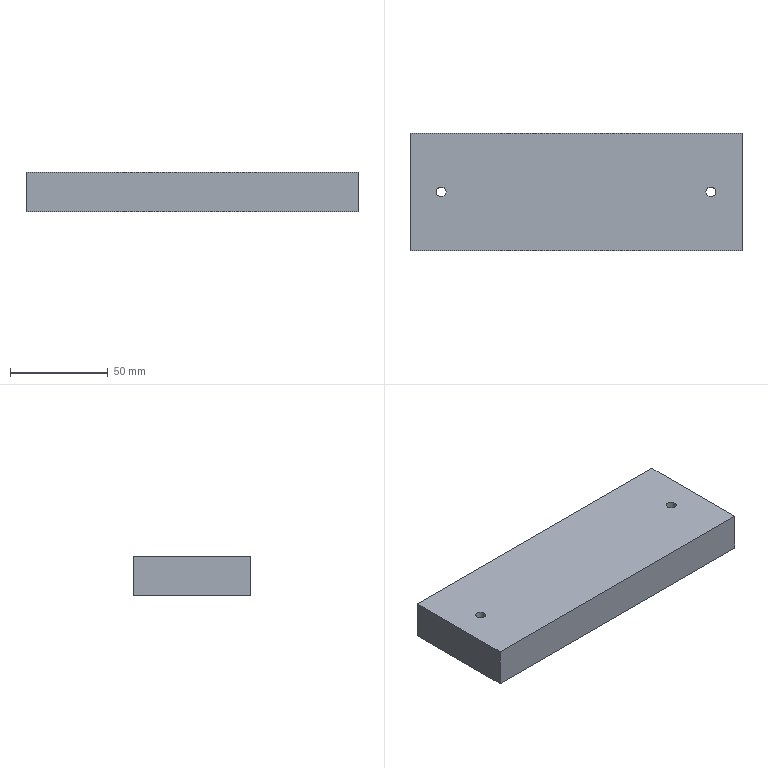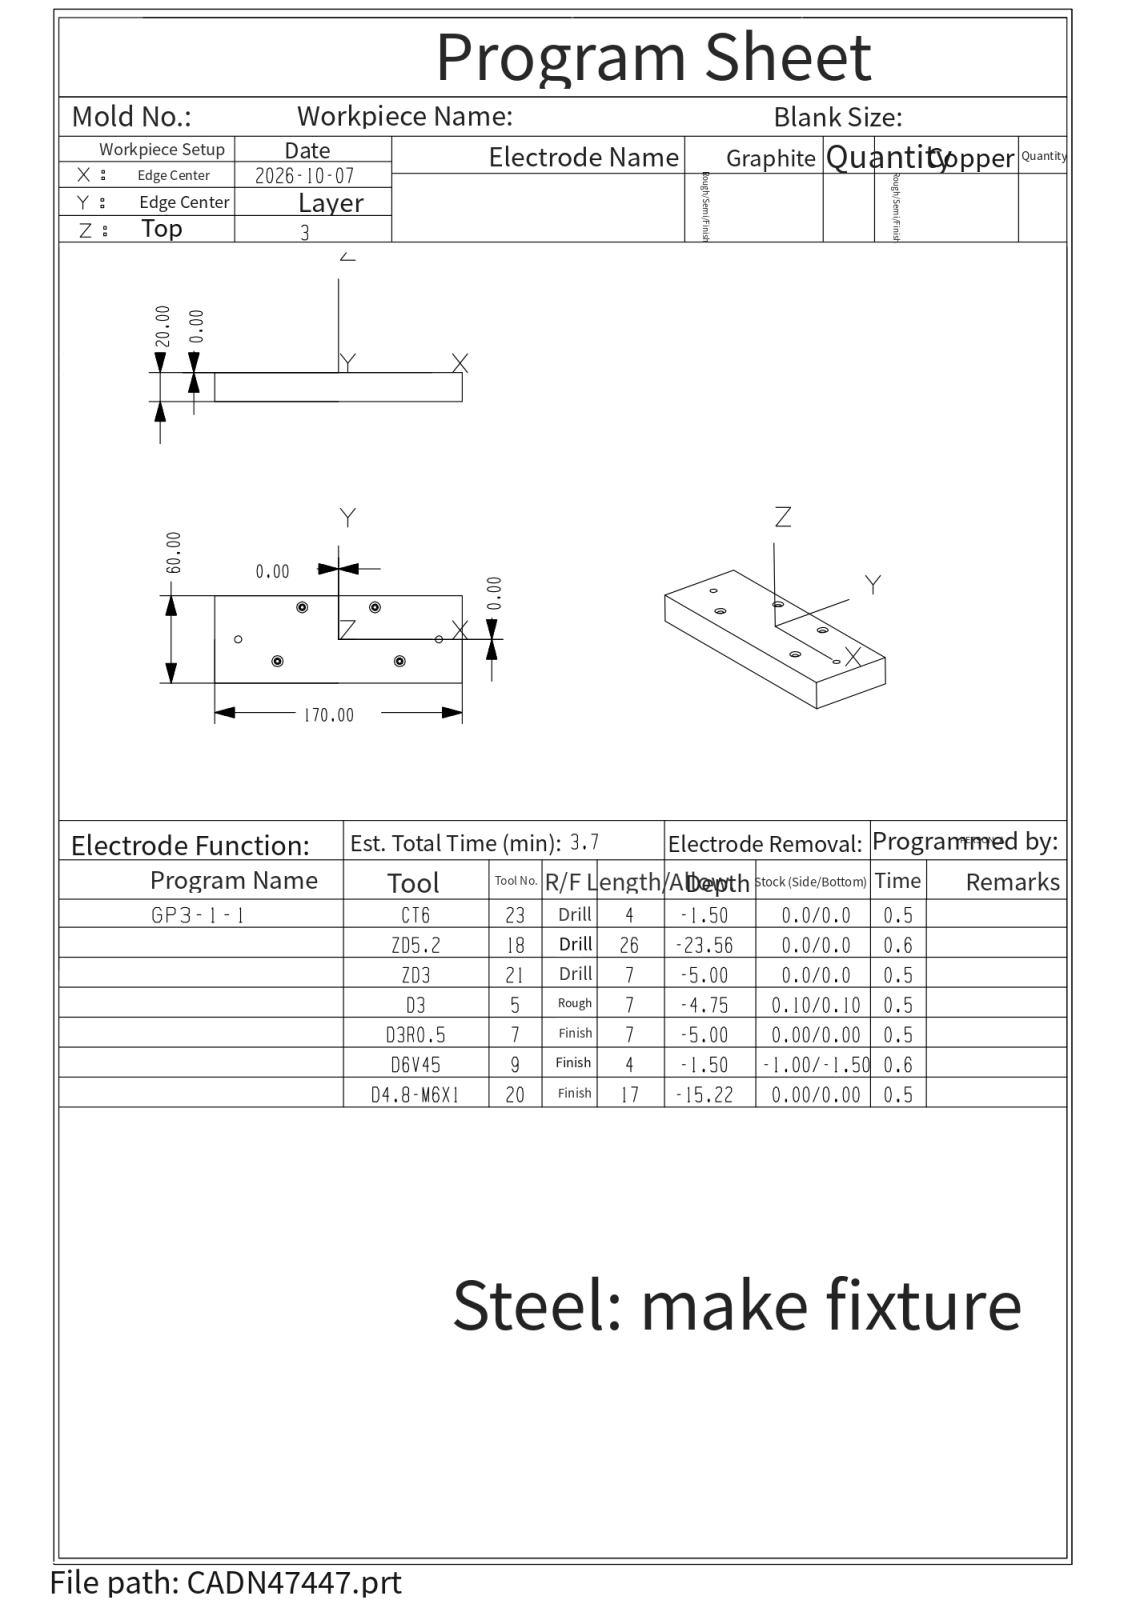NC program | NX | posted by the shop | part box 170 x 60 x 20 mm
Lines 13298 to 14163 of 14163:
T09 M06
T20
( name=D6V45    T=9 )
( XY = -0.50 )
( Z = -1.50 )
G00 G90 G54 X0.0 Y-31.6 S5000 M03
G43 Z10. H09 M08
Z-1.5
G01 X.6 F500.
G03 X0.0 Y-31. I-.6 J0.0
G01 X-84.5 F1000.
G02 X-86. Y-29.5 I0.0 J1.5
G01 Y29.5
G02 X-84.5 Y31. I1.5 J0.0
G01 X84.5
G02 X86. Y29.5 I0.0 J-1.5
G01 Y-29.5
G02 X84.5 Y-31. I-1.5 J0.0
G01 X0.0
G03 X-.6 Y-31.6 I0.0 J-.6
G01 X0.0
G00 Z10.
G00 X68.1 Y0.0 S5000 M03
M08
Z-1.5
G01 Y.6 F500.
G03 X67.5 Y0.0 I0.0 J-.6
I1.5 J0.0 F1000.
X68.1 Y-.6 I.6 J0.0
G01 Y0.0
X67.6
Y.6 F500.
G03 X67. Y0.0 I0.0 J-.6
I2. J0.0 F1000.
X67.6 Y-.6 I.6 J0.0
G01 Y0.0
G00 Z10.
X-69.9
Z-1.5
G01 Y.6 F500.
G03 X-70.5 Y0.0 I0.0 J-.6
I1.5 J0.0 F1000.
X-69.9 Y-.6 I.6 J0.0
G01 Y0.0
X-70.4
Y.6 F500.
G03 X-71. Y0.0 I0.0 J-.6
I2. J0.0 F1000.
X-70.4 Y-.6 I.6 J0.0
G01 Y0.0
G00 Z10.
M05
M09
G91 G28 Z0.0
M01
N07
T20 M06
T23
( name=D4.8-M6X1    T=20 )
( XY = 0.00 )
( Z = -1.50 )
G00 G90 G54 X69. Y0.0 S6000 M03
G43 Z10. H20 M08
Z.218
G01 X69.032 Y.095 F1000.
X69.119 Y.235 Z.174
X69.273 Y.3 Z.131
X69.439 Y.272 Z.087
X69.564 Y.161 Z.044
X69.6 Y0.0 Z0.0
X69.532 Y-.299 Z-.082 F2000.
X69.317 Y-.521 Z-.163
X69.021 Y-.61 Z-.245
X68.719 Y-.542 Z-.326
X68.49 Y-.335 Z-.408
X68.391 Y-.042 Z-.489
X68.449 Y.262 Z-.571
X68.648 Y.498 Z-.652
X68.938 Y.607 Z-.734
X69.243 Y.559 Z-.815
X69.486 Y.369 Z-.897
X69.604 Y.083 Z-.978
X69.567 Y-.224 Z-1.06
X69.385 Y-.473 Z-1.141
X69.104 Y-.601 Z-1.223
X68.796 Y-.575 Z-1.304
X68.54 Y-.401 Z-1.386
X68.403 Y-.124 Z-1.467
X68.419 Y.185 Z-1.549
X68.584 Y.446 Z-1.63
X68.856 Y.593 Z-1.712
X69.165 Y.587 Z-1.793
X69.431 Y.431 Z-1.875
X69.587 Y.165 Z-1.957
X69.593 Y-.144 Z-2.038
X69.446 Y-.416 Z-2.12
X69.185 Y-.581 Z-2.201
X68.876 Y-.597 Z-2.283
X68.599 Y-.46 Z-2.364
X68.425 Y-.204 Z-2.446
X68.399 Y.104 Z-2.527
X68.527 Y.385 Z-2.609
X68.776 Y.567 Z-2.69
X69.083 Y.604 Z-2.772
X69.369 Y.486 Z-2.853
X69.559 Y.243 Z-2.935
X69.607 Y-.062 Z-3.016
X69.498 Y-.352 Z-3.098
X69.262 Y-.551 Z-3.179
X68.958 Y-.609 Z-3.261
X68.665 Y-.51 Z-3.342
X68.458 Y-.281 Z-3.424
X68.39 Y.021 Z-3.505
X68.479 Y.317 Z-3.587
X68.701 Y.532 Z-3.668
X69. Y.61 Z-3.75
X69.299 Y.532 Z-3.832
X69.521 Y.317 Z-3.913
X69.61 Y.021 Z-3.995
X69.542 Y-.281 Z-4.076
X69.335 Y-.51 Z-4.158
X69.042 Y-.609 Z-4.239
X68.738 Y-.551 Z-4.321
X68.502 Y-.352 Z-4.402
X68.393 Y-.062 Z-4.484
X68.441 Y.243 Z-4.565
X68.631 Y.486 Z-4.647
X68.917 Y.604 Z-4.728
X69.224 Y.567 Z-4.81
X69.473 Y.385 Z-4.891
X69.601 Y.104 Z-4.973
X69.575 Y-.204 Z-5.054
X69.401 Y-.46 Z-5.136
X69.124 Y-.597 Z-5.217
X68.815 Y-.581 Z-5.299
X68.554 Y-.416 Z-5.38
X68.407 Y-.144 Z-5.462
X68.413 Y.165 Z-5.543
X68.569 Y.431 Z-5.625
X68.835 Y.587 Z-5.707
X69.144 Y.593 Z-5.788
X69.416 Y.446 Z-5.87
X69.581 Y.185 Z-5.951
X69.597 Y-.124 Z-6.033
X69.46 Y-.401 Z-6.114
X69.204 Y-.575 Z-6.196
X68.896 Y-.601 Z-6.277
X68.615 Y-.473 Z-6.359
X68.433 Y-.224 Z-6.44
X68.396 Y.083 Z-6.522
X68.514 Y.369 Z-6.603
X68.757 Y.559 Z-6.685
X69.062 Y.607 Z-6.766
X69.352 Y.498 Z-6.848
X69.551 Y.262 Z-6.929
X69.609 Y-.042 Z-7.011
X69.51 Y-.335 Z-7.092
X69.281 Y-.542 Z-7.174
X68.979 Y-.61 Z-7.255
X68.683 Y-.521 Z-7.337
X68.468 Y-.299 Z-7.418
X68.39 Y0.0 Z-7.5
X68.468 Y.299 Z-7.582
X68.683 Y.521 Z-7.663
X68.979 Y.61 Z-7.745
X69.281 Y.542 Z-7.826
X69.51 Y.335 Z-7.908
X69.609 Y.042 Z-7.989
X69.551 Y-.262 Z-8.071
X69.352 Y-.498 Z-8.152
X69.062 Y-.607 Z-8.234
X68.757 Y-.559 Z-8.315
X68.514 Y-.369 Z-8.397
X68.396 Y-.083 Z-8.478
X68.433 Y.224 Z-8.56
X68.615 Y.473 Z-8.641
X68.896 Y.601 Z-8.723
X69.204 Y.575 Z-8.804
X69.46 Y.401 Z-8.886
X69.597 Y.124 Z-8.967
X69.581 Y-.185 Z-9.049
X69.416 Y-.446 Z-9.13
X69.144 Y-.593 Z-9.212
X68.835 Y-.587 Z-9.293
X68.569 Y-.431 Z-9.375
X68.413 Y-.165 Z-9.457
X68.407 Y.144 Z-9.538
X68.554 Y.416 Z-9.62
X68.815 Y.581 Z-9.701
X69.124 Y.597 Z-9.783
X69.401 Y.46 Z-9.864
X69.575 Y.204 Z-9.946
X69.601 Y-.104 Z-10.027
X69.473 Y-.385 Z-10.109
X69.224 Y-.567 Z-10.19
X68.917 Y-.604 Z-10.272
X68.631 Y-.486 Z-10.353
X68.441 Y-.243 Z-10.435
X68.393 Y.062 Z-10.516
X68.502 Y.352 Z-10.598
X68.738 Y.551 Z-10.679
X69.042 Y.609 Z-10.761
X69.335 Y.51 Z-10.842
X69.542 Y.281 Z-10.924
X69.61 Y-.021 Z-11.005
X69.521 Y-.317 Z-11.087
X69.299 Y-.532 Z-11.168
X69. Y-.61 Z-11.25
X68.701 Y-.532 Z-11.332
X68.479 Y-.317 Z-11.413
X68.39 Y-.021 Z-11.495
X68.458 Y.281 Z-11.576
X68.665 Y.51 Z-11.658
X68.958 Y.609 Z-11.739
X69.262 Y.551 Z-11.821
X69.498 Y.352 Z-11.902
X69.607 Y.062 Z-11.984
X69.559 Y-.243 Z-12.065
X69.369 Y-.486 Z-12.147
X69.083 Y-.604 Z-12.228
X68.776 Y-.567 Z-12.31
X68.527 Y-.385 Z-12.391
X68.399 Y-.104 Z-12.473
X68.425 Y.204 Z-12.554
X68.599 Y.46 Z-12.636
X68.876 Y.597 Z-12.717
X69.185 Y.581 Z-12.799
X69.446 Y.416 Z-12.88
X69.593 Y.144 Z-12.962
X69.587 Y-.165 Z-13.043
X69.431 Y-.431 Z-13.125
X69.165 Y-.587 Z-13.207
X68.856 Y-.593 Z-13.288
X68.584 Y-.446 Z-13.37
X68.419 Y-.185 Z-13.451
X68.403 Y.124 Z-13.533
X68.54 Y.401 Z-13.614
X68.796 Y.575 Z-13.696
X69.104 Y.601 Z-13.777
X69.385 Y.473 Z-13.859
X69.567 Y.224 Z-13.94
X69.604 Y-.083 Z-14.022
X69.486 Y-.369 Z-14.103
X69.243 Y-.559 Z-14.185
X68.938 Y-.607 Z-14.266
X68.648 Y-.498 Z-14.348
X68.449 Y-.262 Z-14.429
X68.391 Y.042 Z-14.511
X68.49 Y.335 Z-14.592
X68.719 Y.542 Z-14.674
X69.021 Y.61 Z-14.755
X69.317 Y.521 Z-14.837
X69.532 Y.299 Z-14.918
X69.6 Y0.0 Z-15.
X69.564 Y-.161 Z-15.044
X69.439 Y-.272 Z-15.087
X69.273 Y-.3 Z-15.131
X69.119 Y-.235 Z-15.174
X69.032 Y-.095 Z-15.218
X69. Y0.0
G00 Z10.
Z.218
G01 X69.032 Y.095 F1000.
X69.119 Y.235 Z.174
X69.273 Y.3 Z.131
X69.439 Y.272 Z.087
X69.564 Y.161 Z.044
X69.6 Y0.0 Z0.0
X69.532 Y-.299 Z-.082 F2000.
X69.317 Y-.521 Z-.163
X69.021 Y-.61 Z-.245
X68.719 Y-.542 Z-.326
X68.49 Y-.335 Z-.408
X68.391 Y-.042 Z-.489
X68.449 Y.262 Z-.571
X68.648 Y.498 Z-.652
X68.938 Y.607 Z-.734
X69.243 Y.559 Z-.815
X69.486 Y.369 Z-.897
X69.604 Y.083 Z-.978
X69.567 Y-.224 Z-1.06
X69.385 Y-.473 Z-1.141
X69.104 Y-.601 Z-1.223
X68.796 Y-.575 Z-1.304
X68.54 Y-.401 Z-1.386
X68.403 Y-.124 Z-1.467
X68.419 Y.185 Z-1.549
X68.584 Y.446 Z-1.63
X68.856 Y.593 Z-1.712
X69.165 Y.587 Z-1.793
X69.431 Y.431 Z-1.875
X69.587 Y.165 Z-1.957
X69.593 Y-.144 Z-2.038
X69.446 Y-.416 Z-2.12
X69.185 Y-.581 Z-2.201
X68.876 Y-.597 Z-2.283
X68.599 Y-.46 Z-2.364
X68.425 Y-.204 Z-2.446
X68.399 Y.104 Z-2.527
X68.527 Y.385 Z-2.609
X68.776 Y.567 Z-2.69
X69.083 Y.604 Z-2.772
X69.369 Y.486 Z-2.853
X69.559 Y.243 Z-2.935
X69.607 Y-.062 Z-3.016
X69.498 Y-.352 Z-3.098
X69.262 Y-.551 Z-3.179
X68.958 Y-.609 Z-3.261
X68.665 Y-.51 Z-3.342
X68.458 Y-.281 Z-3.424
X68.39 Y.021 Z-3.505
X68.479 Y.317 Z-3.587
X68.701 Y.532 Z-3.668
X69. Y.61 Z-3.75
X69.299 Y.532 Z-3.832
X69.521 Y.317 Z-3.913
X69.61 Y.021 Z-3.995
X69.542 Y-.281 Z-4.076
X69.335 Y-.51 Z-4.158
X69.042 Y-.609 Z-4.239
X68.738 Y-.551 Z-4.321
X68.502 Y-.352 Z-4.402
X68.393 Y-.062 Z-4.484
X68.441 Y.243 Z-4.565
X68.631 Y.486 Z-4.647
X68.917 Y.604 Z-4.728
X69.224 Y.567 Z-4.81
X69.473 Y.385 Z-4.891
X69.601 Y.104 Z-4.973
X69.575 Y-.204 Z-5.054
X69.401 Y-.46 Z-5.136
X69.124 Y-.597 Z-5.217
X68.815 Y-.581 Z-5.299
X68.554 Y-.416 Z-5.38
X68.407 Y-.144 Z-5.462
X68.413 Y.165 Z-5.543
X68.569 Y.431 Z-5.625
X68.835 Y.587 Z-5.707
X69.144 Y.593 Z-5.788
X69.416 Y.446 Z-5.87
X69.581 Y.185 Z-5.951
X69.597 Y-.124 Z-6.033
X69.46 Y-.401 Z-6.114
X69.204 Y-.575 Z-6.196
X68.896 Y-.601 Z-6.277
X68.615 Y-.473 Z-6.359
X68.433 Y-.224 Z-6.44
X68.396 Y.083 Z-6.522
X68.514 Y.369 Z-6.603
X68.757 Y.559 Z-6.685
X69.062 Y.607 Z-6.766
X69.352 Y.498 Z-6.848
X69.551 Y.262 Z-6.929
X69.609 Y-.042 Z-7.011
X69.51 Y-.335 Z-7.092
X69.281 Y-.542 Z-7.174
X68.979 Y-.61 Z-7.255
X68.683 Y-.521 Z-7.337
X68.468 Y-.299 Z-7.418
X68.39 Y0.0 Z-7.5
X68.468 Y.299 Z-7.582
X68.683 Y.521 Z-7.663
X68.979 Y.61 Z-7.745
X69.281 Y.542 Z-7.826
X69.51 Y.335 Z-7.908
X69.609 Y.042 Z-7.989
X69.551 Y-.262 Z-8.071
X69.352 Y-.498 Z-8.152
X69.062 Y-.607 Z-8.234
X68.757 Y-.559 Z-8.315
X68.514 Y-.369 Z-8.397
X68.396 Y-.083 Z-8.478
X68.433 Y.224 Z-8.56
X68.615 Y.473 Z-8.641
X68.896 Y.601 Z-8.723
X69.204 Y.575 Z-8.804
X69.46 Y.401 Z-8.886
X69.597 Y.124 Z-8.967
X69.581 Y-.185 Z-9.049
X69.416 Y-.446 Z-9.13
X69.144 Y-.593 Z-9.212
X68.835 Y-.587 Z-9.293
X68.569 Y-.431 Z-9.375
X68.413 Y-.165 Z-9.457
X68.407 Y.144 Z-9.538
X68.554 Y.416 Z-9.62
X68.815 Y.581 Z-9.701
X69.124 Y.597 Z-9.783
X69.401 Y.46 Z-9.864
X69.575 Y.204 Z-9.946
X69.601 Y-.104 Z-10.027
X69.473 Y-.385 Z-10.109
X69.224 Y-.567 Z-10.19
X68.917 Y-.604 Z-10.272
X68.631 Y-.486 Z-10.353
X68.441 Y-.243 Z-10.435
X68.393 Y.062 Z-10.516
X68.502 Y.352 Z-10.598
X68.738 Y.551 Z-10.679
X69.042 Y.609 Z-10.761
X69.335 Y.51 Z-10.842
X69.542 Y.281 Z-10.924
X69.61 Y-.021 Z-11.005
X69.521 Y-.317 Z-11.087
X69.299 Y-.532 Z-11.168
X69. Y-.61 Z-11.25
X68.701 Y-.532 Z-11.332
X68.479 Y-.317 Z-11.413
X68.39 Y-.021 Z-11.495
X68.458 Y.281 Z-11.576
X68.665 Y.51 Z-11.658
X68.958 Y.609 Z-11.739
X69.262 Y.551 Z-11.821
X69.498 Y.352 Z-11.902
X69.607 Y.062 Z-11.984
X69.559 Y-.243 Z-12.065
X69.369 Y-.486 Z-12.147
X69.083 Y-.604 Z-12.228
X68.776 Y-.567 Z-12.31
X68.527 Y-.385 Z-12.391
X68.399 Y-.104 Z-12.473
X68.425 Y.204 Z-12.554
X68.599 Y.46 Z-12.636
X68.876 Y.597 Z-12.717
X69.185 Y.581 Z-12.799
X69.446 Y.416 Z-12.88
X69.593 Y.144 Z-12.962
X69.587 Y-.165 Z-13.043
X69.431 Y-.431 Z-13.125
X69.165 Y-.587 Z-13.207
X68.856 Y-.593 Z-13.288
X68.584 Y-.446 Z-13.37
X68.419 Y-.185 Z-13.451
X68.403 Y.124 Z-13.533
X68.54 Y.401 Z-13.614
X68.796 Y.575 Z-13.696
X69.104 Y.601 Z-13.777
X69.385 Y.473 Z-13.859
X69.567 Y.224 Z-13.94
X69.604 Y-.083 Z-14.022
X69.486 Y-.369 Z-14.103
X69.243 Y-.559 Z-14.185
X68.938 Y-.607 Z-14.266
X68.648 Y-.498 Z-14.348
X68.449 Y-.262 Z-14.429
X68.391 Y.042 Z-14.511
X68.49 Y.335 Z-14.592
X68.719 Y.542 Z-14.674
X69.021 Y.61 Z-14.755
X69.317 Y.521 Z-14.837
X69.532 Y.299 Z-14.918
X69.6 Y0.0 Z-15.
X69.564 Y-.161 Z-15.044
X69.439 Y-.272 Z-15.087
X69.273 Y-.3 Z-15.131
X69.119 Y-.235 Z-15.174
X69.032 Y-.095 Z-15.218
X69. Y0.0
G00 Z10.
X-69.
Z.218
G01 X-68.968 Y.095 F1000.
X-68.881 Y.235 Z.174
X-68.727 Y.3 Z.131
X-68.561 Y.272 Z.087
X-68.436 Y.161 Z.044
X-68.4 Y0.0 Z0.0
X-68.468 Y-.299 Z-.082 F2000.
X-68.683 Y-.521 Z-.163
X-68.979 Y-.61 Z-.245
X-69.281 Y-.542 Z-.326
X-69.51 Y-.335 Z-.408
X-69.609 Y-.042 Z-.489
X-69.551 Y.262 Z-.571
X-69.352 Y.498 Z-.652
X-69.062 Y.607 Z-.734
X-68.757 Y.559 Z-.815
X-68.514 Y.369 Z-.897
X-68.396 Y.083 Z-.978
X-68.433 Y-.224 Z-1.06
X-68.615 Y-.473 Z-1.141
X-68.896 Y-.601 Z-1.223
X-69.204 Y-.575 Z-1.304
X-69.46 Y-.401 Z-1.386
X-69.597 Y-.124 Z-1.467
X-69.581 Y.185 Z-1.549
X-69.416 Y.446 Z-1.63
X-69.144 Y.593 Z-1.712
X-68.835 Y.587 Z-1.793
X-68.569 Y.431 Z-1.875
X-68.413 Y.165 Z-1.957
X-68.407 Y-.144 Z-2.038
X-68.554 Y-.416 Z-2.12
X-68.815 Y-.581 Z-2.201
X-69.124 Y-.597 Z-2.283
X-69.401 Y-.46 Z-2.364
X-69.575 Y-.204 Z-2.446
X-69.601 Y.104 Z-2.527
X-69.473 Y.385 Z-2.609
X-69.224 Y.567 Z-2.69
X-68.917 Y.604 Z-2.772
X-68.631 Y.486 Z-2.853
X-68.441 Y.243 Z-2.935
X-68.393 Y-.062 Z-3.016
X-68.502 Y-.352 Z-3.098
X-68.738 Y-.551 Z-3.179
X-69.042 Y-.609 Z-3.261
X-69.335 Y-.51 Z-3.342
X-69.542 Y-.281 Z-3.424
X-69.61 Y.021 Z-3.505
X-69.521 Y.317 Z-3.587
X-69.299 Y.532 Z-3.668
X-69. Y.61 Z-3.75
X-68.701 Y.532 Z-3.832
X-68.479 Y.317 Z-3.913
X-68.39 Y.021 Z-3.995
X-68.458 Y-.281 Z-4.076
X-68.665 Y-.51 Z-4.158
X-68.958 Y-.609 Z-4.239
X-69.262 Y-.551 Z-4.321
X-69.498 Y-.352 Z-4.402
X-69.607 Y-.062 Z-4.484
X-69.559 Y.243 Z-4.565
X-69.369 Y.486 Z-4.647
X-69.083 Y.604 Z-4.728
X-68.776 Y.567 Z-4.81
X-68.527 Y.385 Z-4.891
X-68.399 Y.104 Z-4.973
X-68.425 Y-.204 Z-5.054
X-68.599 Y-.46 Z-5.136
X-68.876 Y-.597 Z-5.217
X-69.185 Y-.581 Z-5.299
X-69.446 Y-.416 Z-5.38
X-69.593 Y-.144 Z-5.462
X-69.587 Y.165 Z-5.543
X-69.431 Y.431 Z-5.625
X-69.165 Y.587 Z-5.707
X-68.856 Y.593 Z-5.788
X-68.584 Y.446 Z-5.87
X-68.419 Y.185 Z-5.951
X-68.403 Y-.124 Z-6.033
X-68.54 Y-.401 Z-6.114
X-68.796 Y-.575 Z-6.196
X-69.104 Y-.601 Z-6.277
X-69.385 Y-.473 Z-6.359
X-69.567 Y-.224 Z-6.44
X-69.604 Y.083 Z-6.522
X-69.486 Y.369 Z-6.603
X-69.243 Y.559 Z-6.685
X-68.938 Y.607 Z-6.766
X-68.648 Y.498 Z-6.848
X-68.449 Y.262 Z-6.929
X-68.391 Y-.042 Z-7.011
X-68.49 Y-.335 Z-7.092
X-68.719 Y-.542 Z-7.174
X-69.021 Y-.61 Z-7.255
X-69.317 Y-.521 Z-7.337
X-69.532 Y-.299 Z-7.418
X-69.61 Y0.0 Z-7.5
X-69.532 Y.299 Z-7.582
X-69.317 Y.521 Z-7.663
X-69.021 Y.61 Z-7.745
X-68.719 Y.542 Z-7.826
X-68.49 Y.335 Z-7.908
X-68.391 Y.042 Z-7.989
X-68.449 Y-.262 Z-8.071
X-68.648 Y-.498 Z-8.152
X-68.938 Y-.607 Z-8.234
X-69.243 Y-.559 Z-8.315
X-69.486 Y-.369 Z-8.397
X-69.604 Y-.083 Z-8.478
X-69.567 Y.224 Z-8.56
X-69.385 Y.473 Z-8.641
X-69.104 Y.601 Z-8.723
X-68.796 Y.575 Z-8.804
X-68.54 Y.401 Z-8.886
X-68.403 Y.124 Z-8.967
X-68.419 Y-.185 Z-9.049
X-68.584 Y-.446 Z-9.13
X-68.856 Y-.593 Z-9.212
X-69.165 Y-.587 Z-9.293
X-69.431 Y-.431 Z-9.375
X-69.587 Y-.165 Z-9.457
X-69.593 Y.144 Z-9.538
X-69.446 Y.416 Z-9.62
X-69.185 Y.581 Z-9.701
X-68.876 Y.597 Z-9.783
X-68.599 Y.46 Z-9.864
X-68.425 Y.204 Z-9.946
X-68.399 Y-.104 Z-10.027
X-68.527 Y-.385 Z-10.109
X-68.776 Y-.567 Z-10.19
X-69.083 Y-.604 Z-10.272
X-69.369 Y-.486 Z-10.353
X-69.559 Y-.243 Z-10.435
X-69.607 Y.062 Z-10.516
X-69.498 Y.352 Z-10.598
X-69.262 Y.551 Z-10.679
X-68.958 Y.609 Z-10.761
X-68.665 Y.51 Z-10.842
X-68.458 Y.281 Z-10.924
X-68.39 Y-.021 Z-11.005
X-68.479 Y-.317 Z-11.087
X-68.701 Y-.532 Z-11.168
X-69. Y-.61 Z-11.25
X-69.299 Y-.532 Z-11.332
X-69.521 Y-.317 Z-11.413
X-69.61 Y-.021 Z-11.495
X-69.542 Y.281 Z-11.576
X-69.335 Y.51 Z-11.658
X-69.042 Y.609 Z-11.739
X-68.738 Y.551 Z-11.821
X-68.502 Y.352 Z-11.902
X-68.393 Y.062 Z-11.984
X-68.441 Y-.243 Z-12.065
X-68.631 Y-.486 Z-12.147
X-68.917 Y-.604 Z-12.228
X-69.224 Y-.567 Z-12.31
X-69.473 Y-.385 Z-12.391
X-69.601 Y-.104 Z-12.473
X-69.575 Y.204 Z-12.554
X-69.401 Y.46 Z-12.636
X-69.124 Y.597 Z-12.717
X-68.815 Y.581 Z-12.799
X-68.554 Y.416 Z-12.88
X-68.407 Y.144 Z-12.962
X-68.413 Y-.165 Z-13.043
X-68.569 Y-.431 Z-13.125
X-68.835 Y-.587 Z-13.207
X-69.144 Y-.593 Z-13.288
X-69.416 Y-.446 Z-13.37
X-69.581 Y-.185 Z-13.451
X-69.597 Y.124 Z-13.533
X-69.46 Y.401 Z-13.614
X-69.204 Y.575 Z-13.696
X-68.896 Y.601 Z-13.777
X-68.615 Y.473 Z-13.859
X-68.433 Y.224 Z-13.94
X-68.396 Y-.083 Z-14.022
X-68.514 Y-.369 Z-14.103
X-68.757 Y-.559 Z-14.185
X-69.062 Y-.607 Z-14.266
X-69.352 Y-.498 Z-14.348
X-69.551 Y-.262 Z-14.429
X-69.609 Y.042 Z-14.511
X-69.51 Y.335 Z-14.592
X-69.281 Y.542 Z-14.674
X-68.979 Y.61 Z-14.755
X-68.683 Y.521 Z-14.837
X-68.468 Y.299 Z-14.918
X-68.4 Y0.0 Z-15.
X-68.436 Y-.161 Z-15.044
X-68.561 Y-.272 Z-15.087
X-68.727 Y-.3 Z-15.131
X-68.881 Y-.235 Z-15.174
X-68.968 Y-.095 Z-15.218
X-69. Y0.0
G00 Z10.
Z.218
G01 X-68.968 Y.095 F1000.
X-68.881 Y.235 Z.174
X-68.727 Y.3 Z.131
X-68.561 Y.272 Z.087
X-68.436 Y.161 Z.044
X-68.4 Y0.0 Z0.0
X-68.468 Y-.299 Z-.082 F2000.
X-68.683 Y-.521 Z-.163
X-68.979 Y-.61 Z-.245
X-69.281 Y-.542 Z-.326
X-69.51 Y-.335 Z-.408
X-69.609 Y-.042 Z-.489
X-69.551 Y.262 Z-.571
X-69.352 Y.498 Z-.652
X-69.062 Y.607 Z-.734
X-68.757 Y.559 Z-.815
X-68.514 Y.369 Z-.897
X-68.396 Y.083 Z-.978
X-68.433 Y-.224 Z-1.06
X-68.615 Y-.473 Z-1.141
X-68.896 Y-.601 Z-1.223
X-69.204 Y-.575 Z-1.304
X-69.46 Y-.401 Z-1.386
X-69.597 Y-.124 Z-1.467
X-69.581 Y.185 Z-1.549
X-69.416 Y.446 Z-1.63
X-69.144 Y.593 Z-1.712
X-68.835 Y.587 Z-1.793
X-68.569 Y.431 Z-1.875
X-68.413 Y.165 Z-1.957
X-68.407 Y-.144 Z-2.038
X-68.554 Y-.416 Z-2.12
X-68.815 Y-.581 Z-2.201
X-69.124 Y-.597 Z-2.283
X-69.401 Y-.46 Z-2.364
X-69.575 Y-.204 Z-2.446
X-69.601 Y.104 Z-2.527
X-69.473 Y.385 Z-2.609
X-69.224 Y.567 Z-2.69
X-68.917 Y.604 Z-2.772
X-68.631 Y.486 Z-2.853
X-68.441 Y.243 Z-2.935
X-68.393 Y-.062 Z-3.016
X-68.502 Y-.352 Z-3.098
X-68.738 Y-.551 Z-3.179
X-69.042 Y-.609 Z-3.261
X-69.335 Y-.51 Z-3.342
X-69.542 Y-.281 Z-3.424
X-69.61 Y.021 Z-3.505
X-69.521 Y.317 Z-3.587
X-69.299 Y.532 Z-3.668
X-69. Y.61 Z-3.75
X-68.701 Y.532 Z-3.832
X-68.479 Y.317 Z-3.913
X-68.39 Y.021 Z-3.995
X-68.458 Y-.281 Z-4.076
X-68.665 Y-.51 Z-4.158
X-68.958 Y-.609 Z-4.239
X-69.262 Y-.551 Z-4.321
X-69.498 Y-.352 Z-4.402
X-69.607 Y-.062 Z-4.484
X-69.559 Y.243 Z-4.565
X-69.369 Y.486 Z-4.647
X-69.083 Y.604 Z-4.728
X-68.776 Y.567 Z-4.81
X-68.527 Y.385 Z-4.891
X-68.399 Y.104 Z-4.973
X-68.425 Y-.204 Z-5.054
X-68.599 Y-.46 Z-5.136
X-68.876 Y-.597 Z-5.217
X-69.185 Y-.581 Z-5.299
X-69.446 Y-.416 Z-5.38
X-69.593 Y-.144 Z-5.462
X-69.587 Y.165 Z-5.543
X-69.431 Y.431 Z-5.625
X-69.165 Y.587 Z-5.707
X-68.856 Y.593 Z-5.788
X-68.584 Y.446 Z-5.87
X-68.419 Y.185 Z-5.951
X-68.403 Y-.124 Z-6.033
X-68.54 Y-.401 Z-6.114
X-68.796 Y-.575 Z-6.196
X-69.104 Y-.601 Z-6.277
X-69.385 Y-.473 Z-6.359
X-69.567 Y-.224 Z-6.44
X-69.604 Y.083 Z-6.522
X-69.486 Y.369 Z-6.603
X-69.243 Y.559 Z-6.685
X-68.938 Y.607 Z-6.766
X-68.648 Y.498 Z-6.848
X-68.449 Y.262 Z-6.929
X-68.391 Y-.042 Z-7.011
X-68.49 Y-.335 Z-7.092
X-68.719 Y-.542 Z-7.174
X-69.021 Y-.61 Z-7.255
X-69.317 Y-.521 Z-7.337
X-69.532 Y-.299 Z-7.418
X-69.61 Y0.0 Z-7.5
X-69.532 Y.299 Z-7.582
X-69.317 Y.521 Z-7.663
X-69.021 Y.61 Z-7.745
X-68.719 Y.542 Z-7.826
X-68.49 Y.335 Z-7.908
X-68.391 Y.042 Z-7.989
X-68.449 Y-.262 Z-8.071
X-68.648 Y-.498 Z-8.152
X-68.938 Y-.607 Z-8.234
X-69.243 Y-.559 Z-8.315
X-69.486 Y-.369 Z-8.397
X-69.604 Y-.083 Z-8.478
X-69.567 Y.224 Z-8.56
X-69.385 Y.473 Z-8.641
X-69.104 Y.601 Z-8.723
X-68.796 Y.575 Z-8.804
X-68.54 Y.401 Z-8.886
X-68.403 Y.124 Z-8.967
X-68.419 Y-.185 Z-9.049
X-68.584 Y-.446 Z-9.13
X-68.856 Y-.593 Z-9.212
X-69.165 Y-.587 Z-9.293
X-69.431 Y-.431 Z-9.375
X-69.587 Y-.165 Z-9.457
X-69.593 Y.144 Z-9.538
X-69.446 Y.416 Z-9.62
X-69.185 Y.581 Z-9.701
X-68.876 Y.597 Z-9.783
X-68.599 Y.46 Z-9.864
X-68.425 Y.204 Z-9.946
X-68.399 Y-.104 Z-10.027
X-68.527 Y-.385 Z-10.109
X-68.776 Y-.567 Z-10.19
X-69.083 Y-.604 Z-10.272
X-69.369 Y-.486 Z-10.353
X-69.559 Y-.243 Z-10.435
X-69.607 Y.062 Z-10.516
X-69.498 Y.352 Z-10.598
X-69.262 Y.551 Z-10.679
X-68.958 Y.609 Z-10.761
X-68.665 Y.51 Z-10.842
X-68.458 Y.281 Z-10.924
X-68.39 Y-.021 Z-11.005
X-68.479 Y-.317 Z-11.087
X-68.701 Y-.532 Z-11.168
X-69. Y-.61 Z-11.25
X-69.299 Y-.532 Z-11.332
X-69.521 Y-.317 Z-11.413
X-69.61 Y-.021 Z-11.495
X-69.542 Y.281 Z-11.576
X-69.335 Y.51 Z-11.658
X-69.042 Y.609 Z-11.739
X-68.738 Y.551 Z-11.821
X-68.502 Y.352 Z-11.902
X-68.393 Y.062 Z-11.984
X-68.441 Y-.243 Z-12.065
X-68.631 Y-.486 Z-12.147
X-68.917 Y-.604 Z-12.228
X-69.224 Y-.567 Z-12.31
X-69.473 Y-.385 Z-12.391
X-69.601 Y-.104 Z-12.473
X-69.575 Y.204 Z-12.554
X-69.401 Y.46 Z-12.636
X-69.124 Y.597 Z-12.717
X-68.815 Y.581 Z-12.799
X-68.554 Y.416 Z-12.88
X-68.407 Y.144 Z-12.962
X-68.413 Y-.165 Z-13.043
X-68.569 Y-.431 Z-13.125
X-68.835 Y-.587 Z-13.207
X-69.144 Y-.593 Z-13.288
X-69.416 Y-.446 Z-13.37
X-69.581 Y-.185 Z-13.451
X-69.597 Y.124 Z-13.533
X-69.46 Y.401 Z-13.614
X-69.204 Y.575 Z-13.696
X-68.896 Y.601 Z-13.777
X-68.615 Y.473 Z-13.859
X-68.433 Y.224 Z-13.94
X-68.396 Y-.083 Z-14.022
X-68.514 Y-.369 Z-14.103
X-68.757 Y-.559 Z-14.185
X-69.062 Y-.607 Z-14.266
X-69.352 Y-.498 Z-14.348
X-69.551 Y-.262 Z-14.429
X-69.609 Y.042 Z-14.511
X-69.51 Y.335 Z-14.592
X-69.281 Y.542 Z-14.674
X-68.979 Y.61 Z-14.755
X-68.683 Y.521 Z-14.837
X-68.468 Y.299 Z-14.918
X-68.4 Y0.0 Z-15.
X-68.436 Y-.161 Z-15.044
X-68.561 Y-.272 Z-15.087
X-68.727 Y-.3 Z-15.131
X-68.881 Y-.235 Z-15.174
X-68.968 Y-.095 Z-15.218
X-69. Y0.0
G00 Z10.
M05
M09
G91 G28 Z0.0
G91 G28 Y0.
M30
%
(MaxX = 86. , MinX = -86.)
(MaxY = 31. , MinY = -31.6)
(MaxZ = 10. , MinZ = -15.22)